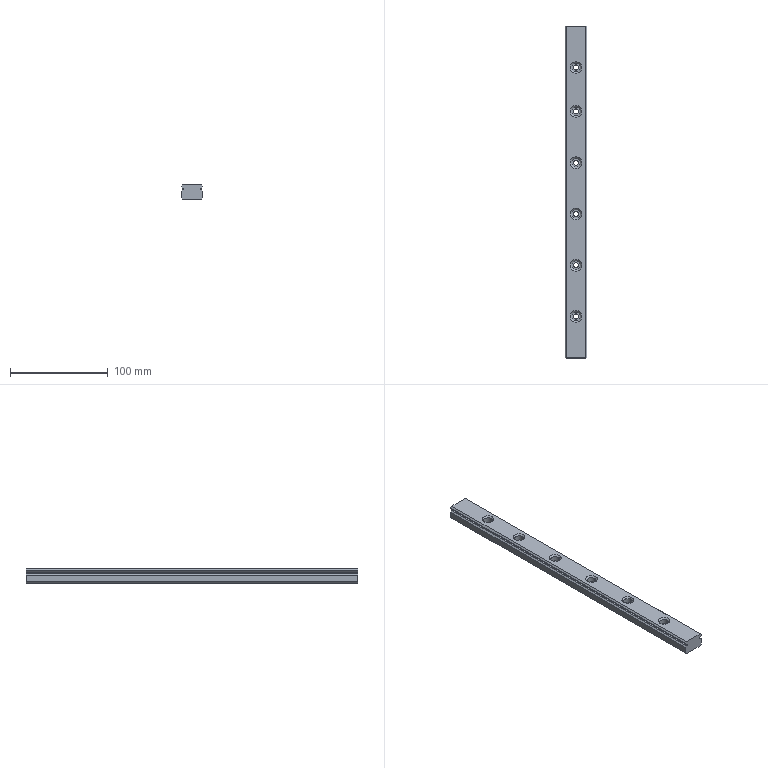Part | STEP file | 1 solid | 76 faces | box 22.5 x 340 x 15 mm | volume 104637 mm3 | plane 28 | cone 24 | cylinder 24 | commonest cylinder face diameters 5.25 x12 9 x12